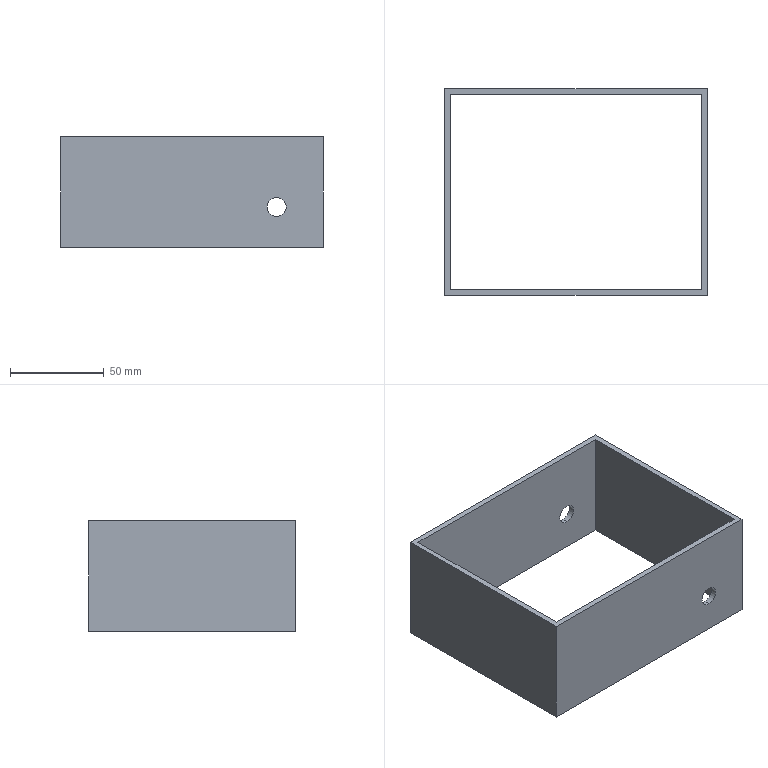Part | SolidWorks | features Extrusion 1, ICE 1 | 1 solid | 14 faces | box 140 x 110 x 59 mm | volume 85886 mm3 | plane 10 | cylinder 4 | commonest cylinder face diameters 10.2 x4
STEP:
#1=CARTESIAN_POINT('',(45.,52.,-13.1));
#2=VERTEX_POINT('',#1);
#3=CARTESIAN_POINT('',(45.,52.,-2.9));
#4=VERTEX_POINT('',#3);
#5=CARTESIAN_POINT('',(45.,52.,-8.));
#6=DIRECTION('',(0.,1.,0.));
#7=DIRECTION('',(0.,0.,1.));
#8=AXIS2_PLACEMENT_3D('',#5,#6,#7);
#9=CIRCLE('',#8,5.1);
#10=EDGE_CURVE('',#2,#4,#9,.T.);
#11=ORIENTED_EDGE('',*,*,#10,.F.);
#12=CARTESIAN_POINT('',(45.,55.,-13.1));
#13=VERTEX_POINT('',#12);
#14=CARTESIAN_POINT('',(45.,-70.,-13.1));
#15=DIRECTION('',(0.,1.,0.));
#16=VECTOR('',#15,1000.);
#17=LINE('',#14,#16);
#18=EDGE_CURVE('',#2,#13,#17,.T.);
#19=ORIENTED_EDGE('',*,*,#18,.T.);
#20=CARTESIAN_POINT('',(45.,55.,-2.9));
#21=VERTEX_POINT('',#20);
#22=CARTESIAN_POINT('',(45.,55.,-8.));
#23=DIRECTION('',(0.,1.,0.));
#24=DIRECTION('',(0.,0.,1.));
#25=AXIS2_PLACEMENT_3D('',#22,#23,#24);
#26=CIRCLE('',#25,5.1);
#27=EDGE_CURVE('',#13,#21,#26,.T.);
#28=ORIENTED_EDGE('',*,*,#27,.T.);
#29=CARTESIAN_POINT('',(45.,-70.,-2.9));
#30=DIRECTION('',(0.,1.,0.));
#31=VECTOR('',#30,1000.);
#32=LINE('',#29,#31);
#33=EDGE_CURVE('',#4,#21,#32,.T.);
#34=ORIENTED_EDGE('',*,*,#33,.F.);
#35=EDGE_LOOP('',(#11,#19,#28,#34));
#36=FACE_OUTER_BOUND('',#35,.T.);
#37=CARTESIAN_POINT('',(45.,-70.,-8.));
#38=DIRECTION('',(0.,1.,0.));
#39=DIRECTION('',(0.,0.,1.));
#40=AXIS2_PLACEMENT_3D('',#37,#38,#39);
#41=CYLINDRICAL_SURFACE('',#40,5.1);
#42=ADVANCED_FACE('',(#36),#41,.F.);
#43=CARTESIAN_POINT('',(45.,-55.,-2.9));
#44=VERTEX_POINT('',#43);
#45=CARTESIAN_POINT('',(45.,-55.,-13.1));
#46=VERTEX_POINT('',#45);
#47=CARTESIAN_POINT('',(45.,-55.,-8.));
#48=DIRECTION('',(0.,-1.,0.));
#49=DIRECTION('',(0.,0.,-1.));
#50=AXIS2_PLACEMENT_3D('',#47,#48,#49);
#51=CIRCLE('',#50,5.1);
#52=EDGE_CURVE('',#44,#46,#51,.T.);
#53=ORIENTED_EDGE('',*,*,#52,.T.);
#54=CARTESIAN_POINT('',(45.,-52.,-13.1));
#55=VERTEX_POINT('',#54);
#56=CARTESIAN_POINT('',(45.,-70.,-13.1));
#57=DIRECTION('',(0.,1.,0.));
#58=VECTOR('',#57,1000.);
#59=LINE('',#56,#58);
#60=EDGE_CURVE('',#46,#55,#59,.T.);
#61=ORIENTED_EDGE('',*,*,#60,.T.);
#62=CARTESIAN_POINT('',(45.,-52.,-2.9));
#63=VERTEX_POINT('',#62);
#64=CARTESIAN_POINT('',(45.,-52.,-8.));
#65=DIRECTION('',(0.,-1.,0.));
#66=DIRECTION('',(0.,0.,-1.));
#67=AXIS2_PLACEMENT_3D('',#64,#65,#66);
#68=CIRCLE('',#67,5.1);
#69=EDGE_CURVE('',#63,#55,#68,.T.);
#70=ORIENTED_EDGE('',*,*,#69,.F.);
#71=CARTESIAN_POINT('',(45.,-70.,-2.9));
#72=DIRECTION('',(0.,1.,0.));
#73=VECTOR('',#72,1000.);
#74=LINE('',#71,#73);
#75=EDGE_CURVE('',#44,#63,#74,.T.);
#76=ORIENTED_EDGE('',*,*,#75,.F.);
#77=EDGE_LOOP('',(#53,#61,#70,#76));
#78=FACE_OUTER_BOUND('',#77,.T.);
#79=CARTESIAN_POINT('',(45.,-70.,-8.));
#80=DIRECTION('',(0.,1.,0.));
#81=DIRECTION('',(0.,0.,1.));
#82=AXIS2_PLACEMENT_3D('',#79,#80,#81);
#83=CYLINDRICAL_SURFACE('',#82,5.1);
#84=ADVANCED_FACE('',(#78),#83,.F.);
#85=CARTESIAN_POINT('',(-70.,55.,29.5));
#86=VERTEX_POINT('',#85);
#87=CARTESIAN_POINT('',(-70.,-55.,29.5));
#88=VERTEX_POINT('',#87);
#89=CARTESIAN_POINT('',(-70.,55.,29.5));
#90=DIRECTION('',(0.,-1.,0.));
#91=VECTOR('',#90,1000.);
#92=LINE('',#89,#91);
#93=EDGE_CURVE('',#86,#88,#92,.T.);
#94=ORIENTED_EDGE('',*,*,#93,.F.);
#95=CARTESIAN_POINT('',(-70.,55.,-29.5));
#96=VERTEX_POINT('',#95);
#97=CARTESIAN_POINT('',(-70.,55.,-29.5));
#98=DIRECTION('',(0.,0.,1.));
#99=VECTOR('',#98,1000.);
#100=LINE('',#97,#99);
#101=EDGE_CURVE('',#96,#86,#100,.T.);
#102=ORIENTED_EDGE('',*,*,#101,.F.);
#103=CARTESIAN_POINT('',(-70.,-55.,-29.5));
#104=VERTEX_POINT('',#103);
#105=CARTESIAN_POINT('',(-70.,55.,-29.5));
#106=DIRECTION('',(0.,-1.,0.));
#107=VECTOR('',#106,1000.);
#108=LINE('',#105,#107);
#109=EDGE_CURVE('',#96,#104,#108,.T.);
#110=ORIENTED_EDGE('',*,*,#109,.T.);
#111=CARTESIAN_POINT('',(-70.,-55.,-29.5));
#112=DIRECTION('',(0.,0.,1.));
#113=VECTOR('',#112,1000.);
#114=LINE('',#111,#113);
#115=EDGE_CURVE('',#104,#88,#114,.T.);
#116=ORIENTED_EDGE('',*,*,#115,.T.);
#117=EDGE_LOOP('',(#94,#102,#110,#116));
#118=FACE_OUTER_BOUND('',#117,.T.);
#119=CARTESIAN_POINT('',(-70.,55.,-29.5));
#120=DIRECTION('',(-1.,0.,0.));
#121=DIRECTION('',(0.,0.,1.));
#122=AXIS2_PLACEMENT_3D('',#119,#120,#121);
#123=PLANE('',#122);
#124=ADVANCED_FACE('',(#118),#123,.T.);
#125=CARTESIAN_POINT('',(45.,55.,-8.));
#126=DIRECTION('',(0.,1.,0.));
#127=DIRECTION('',(0.,0.,1.));
#128=AXIS2_PLACEMENT_3D('',#125,#126,#127);
#129=CIRCLE('',#128,5.1);
#130=EDGE_CURVE('',#21,#13,#129,.T.);
#131=ORIENTED_EDGE('',*,*,#130,.F.);
#132=ORIENTED_EDGE('',*,*,#27,.F.);
#133=EDGE_LOOP('',(#131,#132));
#134=FACE_BOUND('',#133,.T.);
#135=CARTESIAN_POINT('',(70.,55.,29.5));
#136=VERTEX_POINT('',#135);
#137=CARTESIAN_POINT('',(70.,55.,29.5));
#138=DIRECTION('',(-1.,0.,0.));
#139=VECTOR('',#138,1000.);
#140=LINE('',#137,#139);
#141=EDGE_CURVE('',#136,#86,#140,.T.);
#142=ORIENTED_EDGE('',*,*,#141,.F.);
#143=CARTESIAN_POINT('',(70.,55.,-29.5));
#144=VERTEX_POINT('',#143);
#145=CARTESIAN_POINT('',(70.,55.,-29.5));
#146=DIRECTION('',(0.,0.,1.));
#147=VECTOR('',#146,1000.);
#148=LINE('',#145,#147);
#149=EDGE_CURVE('',#144,#136,#148,.T.);
#150=ORIENTED_EDGE('',*,*,#149,.F.);
#151=CARTESIAN_POINT('',(70.,55.,-29.5));
#152=DIRECTION('',(-1.,0.,0.));
#153=VECTOR('',#152,1000.);
#154=LINE('',#151,#153);
#155=EDGE_CURVE('',#144,#96,#154,.T.);
#156=ORIENTED_EDGE('',*,*,#155,.T.);
#157=ORIENTED_EDGE('',*,*,#101,.T.);
#158=EDGE_LOOP('',(#142,#150,#156,#157));
#159=FACE_OUTER_BOUND('',#158,.T.);
#160=CARTESIAN_POINT('',(70.,55.,-29.5));
#161=DIRECTION('',(0.,1.,0.));
#162=DIRECTION('',(0.,0.,1.));
#163=AXIS2_PLACEMENT_3D('',#160,#161,#162);
#164=PLANE('',#163);
#165=ADVANCED_FACE('',(#134,#159),#164,.T.);
#166=CARTESIAN_POINT('',(70.,-55.,29.5));
#167=VERTEX_POINT('',#166);
#168=CARTESIAN_POINT('',(70.,-55.,29.5));
#169=DIRECTION('',(0.,1.,0.));
#170=VECTOR('',#169,1000.);
#171=LINE('',#168,#170);
#172=EDGE_CURVE('',#167,#136,#171,.T.);
#173=ORIENTED_EDGE('',*,*,#172,.F.);
#174=CARTESIAN_POINT('',(70.,-55.,-29.5));
#175=VERTEX_POINT('',#174);
#176=CARTESIAN_POINT('',(70.,-55.,-29.5));
#177=DIRECTION('',(0.,0.,1.));
#178=VECTOR('',#177,1000.);
#179=LINE('',#176,#178);
#180=EDGE_CURVE('',#175,#167,#179,.T.);
#181=ORIENTED_EDGE('',*,*,#180,.F.);
#182=CARTESIAN_POINT('',(70.,-55.,-29.5));
#183=DIRECTION('',(0.,1.,0.));
#184=VECTOR('',#183,1000.);
#185=LINE('',#182,#184);
#186=EDGE_CURVE('',#175,#144,#185,.T.);
#187=ORIENTED_EDGE('',*,*,#186,.T.);
#188=ORIENTED_EDGE('',*,*,#149,.T.);
#189=EDGE_LOOP('',(#173,#181,#187,#188));
#190=FACE_OUTER_BOUND('',#189,.T.);
#191=CARTESIAN_POINT('',(70.,-55.,-29.5));
#192=DIRECTION('',(1.,0.,0.));
#193=DIRECTION('',(0.,0.,-1.));
#194=AXIS2_PLACEMENT_3D('',#191,#192,#193);
#195=PLANE('',#194);
#196=ADVANCED_FACE('',(#190),#195,.T.);
#197=ORIENTED_EDGE('',*,*,#52,.F.);
#198=CARTESIAN_POINT('',(45.,-55.,-8.));
#199=DIRECTION('',(0.,-1.,0.));
#200=DIRECTION('',(0.,0.,-1.));
#201=AXIS2_PLACEMENT_3D('',#198,#199,#200);
#202=CIRCLE('',#201,5.1);
#203=EDGE_CURVE('',#46,#44,#202,.T.);
#204=ORIENTED_EDGE('',*,*,#203,.F.);
#205=EDGE_LOOP('',(#197,#204));
#206=FACE_BOUND('',#205,.T.);
#207=CARTESIAN_POINT('',(-70.,-55.,29.5));
#208=DIRECTION('',(1.,0.,0.));
#209=VECTOR('',#208,1000.);
#210=LINE('',#207,#209);
#211=EDGE_CURVE('',#88,#167,#210,.T.);
#212=ORIENTED_EDGE('',*,*,#211,.F.);
#213=ORIENTED_EDGE('',*,*,#115,.F.);
#214=CARTESIAN_POINT('',(-70.,-55.,-29.5));
#215=DIRECTION('',(1.,0.,0.));
#216=VECTOR('',#215,1000.);
#217=LINE('',#214,#216);
#218=EDGE_CURVE('',#104,#175,#217,.T.);
#219=ORIENTED_EDGE('',*,*,#218,.T.);
#220=ORIENTED_EDGE('',*,*,#180,.T.);
#221=EDGE_LOOP('',(#212,#213,#219,#220));
#222=FACE_OUTER_BOUND('',#221,.T.);
#223=CARTESIAN_POINT('',(-70.,-55.,-29.5));
#224=DIRECTION('',(0.,-1.,0.));
#225=DIRECTION('',(0.,0.,-1.));
#226=AXIS2_PLACEMENT_3D('',#223,#224,#225);
#227=PLANE('',#226);
#228=ADVANCED_FACE('',(#206,#222),#227,.T.);
#229=CARTESIAN_POINT('',(67.,52.,-29.5));
#230=VERTEX_POINT('',#229);
#231=CARTESIAN_POINT('',(-67.,52.,-29.5));
#232=VERTEX_POINT('',#231);
#233=CARTESIAN_POINT('',(67.,52.,-29.5));
#234=DIRECTION('',(-1.,0.,0.));
#235=VECTOR('',#234,1000.);
#236=LINE('',#233,#235);
#237=EDGE_CURVE('',#230,#232,#236,.T.);
#238=ORIENTED_EDGE('',*,*,#237,.T.);
#239=CARTESIAN_POINT('',(-67.,-52.,-29.5));
#240=VERTEX_POINT('',#239);
#241=CARTESIAN_POINT('',(-67.,52.,-29.5));
#242=DIRECTION('',(0.,-1.,0.));
#243=VECTOR('',#242,1000.);
#244=LINE('',#241,#243);
#245=EDGE_CURVE('',#232,#240,#244,.T.);
#246=ORIENTED_EDGE('',*,*,#245,.T.);
#247=CARTESIAN_POINT('',(67.,-52.,-29.5));
#248=VERTEX_POINT('',#247);
#249=CARTESIAN_POINT('',(-67.,-52.,-29.5));
#250=DIRECTION('',(1.,0.,0.));
#251=VECTOR('',#250,1000.);
#252=LINE('',#249,#251);
#253=EDGE_CURVE('',#240,#248,#252,.T.);
#254=ORIENTED_EDGE('',*,*,#253,.T.);
#255=CARTESIAN_POINT('',(67.,-52.,-29.5));
#256=DIRECTION('',(0.,1.,0.));
#257=VECTOR('',#256,1000.);
#258=LINE('',#255,#257);
#259=EDGE_CURVE('',#248,#230,#258,.T.);
#260=ORIENTED_EDGE('',*,*,#259,.T.);
#261=EDGE_LOOP('',(#238,#246,#254,#260));
#262=FACE_BOUND('',#261,.T.);
#263=ORIENTED_EDGE('',*,*,#109,.F.);
#264=ORIENTED_EDGE('',*,*,#155,.F.);
#265=ORIENTED_EDGE('',*,*,#186,.F.);
#266=ORIENTED_EDGE('',*,*,#218,.F.);
#267=EDGE_LOOP('',(#263,#264,#265,#266));
#268=FACE_OUTER_BOUND('',#267,.T.);
#269=CARTESIAN_POINT('',(0.,0.,-29.5));
#270=DIRECTION('',(0.,0.,1.));
#271=DIRECTION('',(1.,0.,0.));
#272=AXIS2_PLACEMENT_3D('',#269,#270,#271);
#273=PLANE('',#272);
#274=ADVANCED_FACE('',(#262,#268),#273,.F.);
#275=CARTESIAN_POINT('',(-67.,52.,29.5));
#276=VERTEX_POINT('',#275);
#277=CARTESIAN_POINT('',(-67.,-52.,29.5));
#278=VERTEX_POINT('',#277);
#279=CARTESIAN_POINT('',(-67.,52.,29.5));
#280=DIRECTION('',(0.,-1.,0.));
#281=VECTOR('',#280,1000.);
#282=LINE('',#279,#281);
#283=EDGE_CURVE('',#276,#278,#282,.T.);
#284=ORIENTED_EDGE('',*,*,#283,.F.);
#285=CARTESIAN_POINT('',(67.,52.,29.5));
#286=VERTEX_POINT('',#285);
#287=CARTESIAN_POINT('',(67.,52.,29.5));
#288=DIRECTION('',(-1.,0.,0.));
#289=VECTOR('',#288,1000.);
#290=LINE('',#287,#289);
#291=EDGE_CURVE('',#286,#276,#290,.T.);
#292=ORIENTED_EDGE('',*,*,#291,.F.);
#293=CARTESIAN_POINT('',(67.,-52.,29.5));
#294=VERTEX_POINT('',#293);
#295=CARTESIAN_POINT('',(67.,-52.,29.5));
#296=DIRECTION('',(0.,1.,0.));
#297=VECTOR('',#296,1000.);
#298=LINE('',#295,#297);
#299=EDGE_CURVE('',#294,#286,#298,.T.);
#300=ORIENTED_EDGE('',*,*,#299,.F.);
#301=CARTESIAN_POINT('',(-67.,-52.,29.5));
#302=DIRECTION('',(1.,0.,0.));
#303=VECTOR('',#302,1000.);
#304=LINE('',#301,#303);
#305=EDGE_CURVE('',#278,#294,#304,.T.);
#306=ORIENTED_EDGE('',*,*,#305,.F.);
#307=EDGE_LOOP('',(#284,#292,#300,#306));
#308=FACE_BOUND('',#307,.T.);
#309=ORIENTED_EDGE('',*,*,#93,.T.);
#310=ORIENTED_EDGE('',*,*,#211,.T.);
#311=ORIENTED_EDGE('',*,*,#172,.T.);
#312=ORIENTED_EDGE('',*,*,#141,.T.);
#313=EDGE_LOOP('',(#309,#310,#311,#312));
#314=FACE_OUTER_BOUND('',#313,.T.);
#315=CARTESIAN_POINT('',(0.,0.,29.5));
#316=DIRECTION('',(0.,0.,1.));
#317=DIRECTION('',(1.,0.,0.));
#318=AXIS2_PLACEMENT_3D('',#315,#316,#317);
#319=PLANE('',#318);
#320=ADVANCED_FACE('',(#308,#314),#319,.T.);
#321=ORIENTED_EDGE('',*,*,#283,.T.);
#322=CARTESIAN_POINT('',(-67.,-52.,-29.5));
#323=DIRECTION('',(0.,0.,1.));
#324=VECTOR('',#323,1000.);
#325=LINE('',#322,#324);
#326=EDGE_CURVE('',#240,#278,#325,.T.);
#327=ORIENTED_EDGE('',*,*,#326,.F.);
#328=ORIENTED_EDGE('',*,*,#245,.F.);
#329=CARTESIAN_POINT('',(-67.,52.,-29.5));
#330=DIRECTION('',(0.,0.,1.));
#331=VECTOR('',#330,1000.);
#332=LINE('',#329,#331);
#333=EDGE_CURVE('',#232,#276,#332,.T.);
#334=ORIENTED_EDGE('',*,*,#333,.T.);
#335=EDGE_LOOP('',(#321,#327,#328,#334));
#336=FACE_OUTER_BOUND('',#335,.T.);
#337=CARTESIAN_POINT('',(-67.,52.,-29.5));
#338=DIRECTION('',(-1.,0.,0.));
#339=DIRECTION('',(0.,0.,1.));
#340=AXIS2_PLACEMENT_3D('',#337,#338,#339);
#341=PLANE('',#340);
#342=ADVANCED_FACE('',(#336),#341,.F.);
#343=CARTESIAN_POINT('',(45.,52.,-8.));
#344=DIRECTION('',(0.,1.,0.));
#345=DIRECTION('',(0.,0.,1.));
#346=AXIS2_PLACEMENT_3D('',#343,#344,#345);
#347=CIRCLE('',#346,5.1);
#348=EDGE_CURVE('',#4,#2,#347,.T.);
#349=ORIENTED_EDGE('',*,*,#348,.T.);
#350=ORIENTED_EDGE('',*,*,#10,.T.);
#351=EDGE_LOOP('',(#349,#350));
#352=FACE_BOUND('',#351,.T.);
#353=ORIENTED_EDGE('',*,*,#291,.T.);
#354=ORIENTED_EDGE('',*,*,#333,.F.);
#355=ORIENTED_EDGE('',*,*,#237,.F.);
#356=CARTESIAN_POINT('',(67.,52.,-29.5));
#357=DIRECTION('',(0.,0.,1.));
#358=VECTOR('',#357,1000.);
#359=LINE('',#356,#358);
#360=EDGE_CURVE('',#230,#286,#359,.T.);
#361=ORIENTED_EDGE('',*,*,#360,.T.);
#362=EDGE_LOOP('',(#353,#354,#355,#361));
#363=FACE_OUTER_BOUND('',#362,.T.);
#364=CARTESIAN_POINT('',(67.,52.,-29.5));
#365=DIRECTION('',(0.,1.,0.));
#366=DIRECTION('',(0.,0.,1.));
#367=AXIS2_PLACEMENT_3D('',#364,#365,#366);
#368=PLANE('',#367);
#369=ADVANCED_FACE('',(#352,#363),#368,.F.);
#370=ORIENTED_EDGE('',*,*,#299,.T.);
#371=ORIENTED_EDGE('',*,*,#360,.F.);
#372=ORIENTED_EDGE('',*,*,#259,.F.);
#373=CARTESIAN_POINT('',(67.,-52.,-29.5));
#374=DIRECTION('',(0.,0.,1.));
#375=VECTOR('',#374,1000.);
#376=LINE('',#373,#375);
#377=EDGE_CURVE('',#248,#294,#376,.T.);
#378=ORIENTED_EDGE('',*,*,#377,.T.);
#379=EDGE_LOOP('',(#370,#371,#372,#378));
#380=FACE_OUTER_BOUND('',#379,.T.);
#381=CARTESIAN_POINT('',(67.,-52.,-29.5));
#382=DIRECTION('',(1.,0.,0.));
#383=DIRECTION('',(0.,0.,-1.));
#384=AXIS2_PLACEMENT_3D('',#381,#382,#383);
#385=PLANE('',#384);
#386=ADVANCED_FACE('',(#380),#385,.F.);
#387=ORIENTED_EDGE('',*,*,#69,.T.);
#388=CARTESIAN_POINT('',(45.,-52.,-8.));
#389=DIRECTION('',(0.,-1.,0.));
#390=DIRECTION('',(0.,0.,-1.));
#391=AXIS2_PLACEMENT_3D('',#388,#389,#390);
#392=CIRCLE('',#391,5.1);
#393=EDGE_CURVE('',#55,#63,#392,.T.);
#394=ORIENTED_EDGE('',*,*,#393,.T.);
#395=EDGE_LOOP('',(#387,#394));
#396=FACE_BOUND('',#395,.T.);
#397=ORIENTED_EDGE('',*,*,#305,.T.);
#398=ORIENTED_EDGE('',*,*,#377,.F.);
#399=ORIENTED_EDGE('',*,*,#253,.F.);
#400=ORIENTED_EDGE('',*,*,#326,.T.);
#401=EDGE_LOOP('',(#397,#398,#399,#400));
#402=FACE_OUTER_BOUND('',#401,.T.);
#403=CARTESIAN_POINT('',(-67.,-52.,-29.5));
#404=DIRECTION('',(0.,-1.,0.));
#405=DIRECTION('',(0.,0.,-1.));
#406=AXIS2_PLACEMENT_3D('',#403,#404,#405);
#407=PLANE('',#406);
#408=ADVANCED_FACE('',(#396,#402),#407,.F.);
#409=ORIENTED_EDGE('',*,*,#60,.F.);
#410=ORIENTED_EDGE('',*,*,#203,.T.);
#411=ORIENTED_EDGE('',*,*,#75,.T.);
#412=ORIENTED_EDGE('',*,*,#393,.F.);
#413=EDGE_LOOP('',(#409,#410,#411,#412));
#414=FACE_OUTER_BOUND('',#413,.T.);
#415=CARTESIAN_POINT('',(45.,-70.,-8.));
#416=DIRECTION('',(0.,1.,0.));
#417=DIRECTION('',(0.,0.,1.));
#418=AXIS2_PLACEMENT_3D('',#415,#416,#417);
#419=CYLINDRICAL_SURFACE('',#418,5.1);
#420=ADVANCED_FACE('',(#414),#419,.F.);
#421=ORIENTED_EDGE('',*,*,#18,.F.);
#422=ORIENTED_EDGE('',*,*,#348,.F.);
#423=ORIENTED_EDGE('',*,*,#33,.T.);
#424=ORIENTED_EDGE('',*,*,#130,.T.);
#425=EDGE_LOOP('',(#421,#422,#423,#424));
#426=FACE_OUTER_BOUND('',#425,.T.);
#427=CARTESIAN_POINT('',(45.,-70.,-8.));
#428=DIRECTION('',(0.,1.,0.));
#429=DIRECTION('',(0.,0.,1.));
#430=AXIS2_PLACEMENT_3D('',#427,#428,#429);
#431=CYLINDRICAL_SURFACE('',#430,5.1);
#432=ADVANCED_FACE('',(#426),#431,.F.);
#433=CLOSED_SHELL('',(#42,#84,#124,#165,#196,#228,#274,#320,#342,#369,#386,#408,#420,#432));
#434=MANIFOLD_SOLID_BREP('',#433);
#435=CARTESIAN_POINT('',(0.,0.,0.));
#436=DIRECTION('',(0.,0.,1.));
#437=DIRECTION('',(1.,0.,0.));
#438=AXIS2_PLACEMENT_3D('',#435,#436,#437);
#439=(LENGTH_UNIT()NAMED_UNIT(*)SI_UNIT(.MILLI.,.METRE.));
#440=UNCERTAINTY_MEASURE_WITH_UNIT(LENGTH_MEASURE(0.00001),#439,'','');
#441=(NAMED_UNIT(*)PLANE_ANGLE_UNIT()SI_UNIT($,.RADIAN.));
#442=(NAMED_UNIT(*)SI_UNIT($,.STERADIAN.)SOLID_ANGLE_UNIT());
#443=(GEOMETRIC_REPRESENTATION_CONTEXT(3)GLOBAL_UNCERTAINTY_ASSIGNED_CONTEXT((#440))GLOBAL_UNIT_ASSIGNED_CONTEXT((#439,#441,#442))REPRESENTATION_CONTEXT('',''));
#444=ADVANCED_BREP_SHAPE_REPRESENTATION('',(#434,#438),#443);